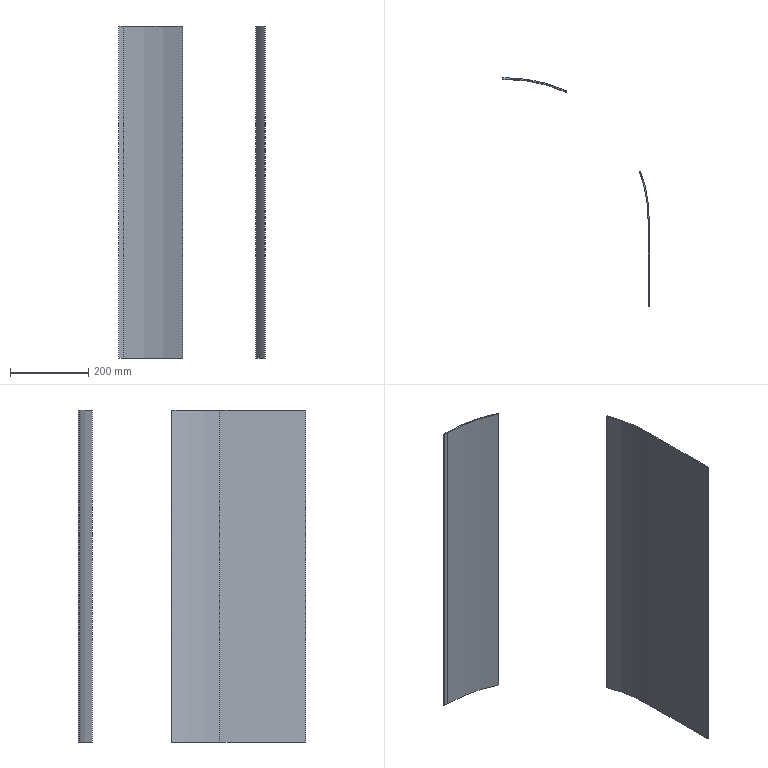Part | NX | features BREP 2, DATUM_CSYS 1, SKETCH 1 | 2 solids | 16 faces | box 375 x 583 x 850 mm | volume 1310584 mm3 | plane 12 | cylinder 4 | commonest cylinder face diameters 720 x2 726 x2
STEP:
#1=CARTESIAN_POINT('',(1041.108,124.153,-31.));
#2=VERTEX_POINT('',#1);
#3=CARTESIAN_POINT('',(1041.108,124.153,819.));
#4=VERTEX_POINT('',#3);
#5=CARTESIAN_POINT('',(1041.108,124.153,-31.));
#6=DIRECTION('',(0.,0.,1.));
#7=VECTOR('',#6,1000.);
#8=LINE('',#5,#7);
#9=EDGE_CURVE('',#2,#4,#8,.T.);
#10=ORIENTED_EDGE('',*,*,#9,.T.);
#11=CARTESIAN_POINT('',(1063.,0.,819.));
#12=VERTEX_POINT('',#11);
#13=CARTESIAN_POINT('',(700.,0.,819.));
#14=DIRECTION('',(0.,0.,-1.));
#15=DIRECTION('',(1.,0.,0.));
#16=AXIS2_PLACEMENT_3D('',#13,#14,#15);
#17=CIRCLE('',#16,363.);
#18=EDGE_CURVE('',#4,#12,#17,.T.);
#19=ORIENTED_EDGE('',*,*,#18,.T.);
#20=CARTESIAN_POINT('',(1063.,0.,-31.));
#21=VERTEX_POINT('',#20);
#22=CARTESIAN_POINT('',(1063.,0.,819.));
#23=DIRECTION('',(0.,0.,-1.));
#24=VECTOR('',#23,1000.);
#25=LINE('',#22,#24);
#26=EDGE_CURVE('',#12,#21,#25,.T.);
#27=ORIENTED_EDGE('',*,*,#26,.T.);
#28=CARTESIAN_POINT('',(700.,0.,-31.));
#29=DIRECTION('',(0.,0.,-1.));
#30=DIRECTION('',(1.,0.,0.));
#31=AXIS2_PLACEMENT_3D('',#28,#29,#30);
#32=CIRCLE('',#31,363.);
#33=EDGE_CURVE('',#2,#21,#32,.T.);
#34=ORIENTED_EDGE('',*,*,#33,.F.);
#35=EDGE_LOOP('',(#10,#19,#27,#34));
#36=FACE_BOUND('',#35,.T.);
#37=CARTESIAN_POINT('',(700.,0.,819.));
#38=DIRECTION('',(0.,0.,-1.));
#39=DIRECTION('',(1.,0.,0.));
#40=AXIS2_PLACEMENT_3D('',#37,#38,#39);
#41=CYLINDRICAL_SURFACE('',#40,363.);
#42=ADVANCED_FACE('',(#36),#41,.T.);
#43=CARTESIAN_POINT('',(1038.289,123.127,819.));
#44=VERTEX_POINT('',#43);
#45=CARTESIAN_POINT('',(1060.,0.,819.));
#46=VERTEX_POINT('',#45);
#47=CARTESIAN_POINT('',(700.,0.,819.));
#48=DIRECTION('',(0.,0.,-1.));
#49=DIRECTION('',(1.,0.,0.));
#50=AXIS2_PLACEMENT_3D('',#47,#48,#49);
#51=CIRCLE('',#50,360.);
#52=EDGE_CURVE('',#44,#46,#51,.T.);
#53=ORIENTED_EDGE('',*,*,#52,.F.);
#54=CARTESIAN_POINT('',(1038.289,123.127,-31.));
#55=VERTEX_POINT('',#54);
#56=CARTESIAN_POINT('',(1038.289,123.127,-31.));
#57=DIRECTION('',(0.,0.,1.));
#58=VECTOR('',#57,1000.);
#59=LINE('',#56,#58);
#60=EDGE_CURVE('',#55,#44,#59,.T.);
#61=ORIENTED_EDGE('',*,*,#60,.F.);
#62=CARTESIAN_POINT('',(1060.,0.,-31.));
#63=VERTEX_POINT('',#62);
#64=CARTESIAN_POINT('',(700.,0.,-31.));
#65=DIRECTION('',(0.,0.,-1.));
#66=DIRECTION('',(1.,0.,0.));
#67=AXIS2_PLACEMENT_3D('',#64,#65,#66);
#68=CIRCLE('',#67,360.);
#69=EDGE_CURVE('',#55,#63,#68,.T.);
#70=ORIENTED_EDGE('',*,*,#69,.T.);
#71=CARTESIAN_POINT('',(1060.,0.,819.));
#72=DIRECTION('',(0.,0.,-1.));
#73=VECTOR('',#72,1000.);
#74=LINE('',#71,#73);
#75=EDGE_CURVE('',#46,#63,#74,.T.);
#76=ORIENTED_EDGE('',*,*,#75,.F.);
#77=EDGE_LOOP('',(#53,#61,#70,#76));
#78=FACE_BOUND('',#77,.T.);
#79=CARTESIAN_POINT('',(700.,0.,819.));
#80=DIRECTION('',(0.,0.,-1.));
#81=DIRECTION('',(1.,0.,0.));
#82=AXIS2_PLACEMENT_3D('',#79,#80,#81);
#83=CYLINDRICAL_SURFACE('',#82,360.);
#84=ADVANCED_FACE('',(#78),#83,.F.);
#85=CARTESIAN_POINT('',(1041.108,124.153,819.));
#86=DIRECTION('',(0.9397,0.342,0.));
#87=VECTOR('',#86,1000.);
#88=LINE('',#85,#87);
#89=EDGE_CURVE('',#44,#4,#88,.T.);
#90=ORIENTED_EDGE('',*,*,#89,.F.);
#91=ORIENTED_EDGE('',*,*,#52,.T.);
#92=CARTESIAN_POINT('',(1060.,-220.,819.));
#93=VERTEX_POINT('',#92);
#94=CARTESIAN_POINT('',(1060.,0.,819.));
#95=DIRECTION('',(0.,-1.,0.));
#96=VECTOR('',#95,1000.);
#97=LINE('',#94,#96);
#98=EDGE_CURVE('',#46,#93,#97,.T.);
#99=ORIENTED_EDGE('',*,*,#98,.T.);
#100=CARTESIAN_POINT('',(1063.,-220.,819.));
#101=VERTEX_POINT('',#100);
#102=CARTESIAN_POINT('',(1063.,-220.,819.));
#103=DIRECTION('',(-1.,0.,0.));
#104=VECTOR('',#103,1000.);
#105=LINE('',#102,#104);
#106=EDGE_CURVE('',#101,#93,#105,.T.);
#107=ORIENTED_EDGE('',*,*,#106,.F.);
#108=CARTESIAN_POINT('',(1063.,0.,819.));
#109=DIRECTION('',(0.,-1.,0.));
#110=VECTOR('',#109,1000.);
#111=LINE('',#108,#110);
#112=EDGE_CURVE('',#12,#101,#111,.T.);
#113=ORIENTED_EDGE('',*,*,#112,.F.);
#114=ORIENTED_EDGE('',*,*,#18,.F.);
#115=EDGE_LOOP('',(#90,#91,#99,#107,#113,#114));
#116=FACE_BOUND('',#115,.T.);
#117=CARTESIAN_POINT('',(700.,0.,819.));
#118=DIRECTION('',(0.,0.,1.));
#119=DIRECTION('',(-1.,0.,0.));
#120=AXIS2_PLACEMENT_3D('',#117,#118,#119);
#121=PLANE('',#120);
#122=ADVANCED_FACE('',(#116),#121,.T.);
#123=ORIENTED_EDGE('',*,*,#69,.F.);
#124=CARTESIAN_POINT('',(1041.108,124.153,-31.));
#125=DIRECTION('',(0.9397,0.342,0.));
#126=VECTOR('',#125,1000.);
#127=LINE('',#124,#126);
#128=EDGE_CURVE('',#55,#2,#127,.T.);
#129=ORIENTED_EDGE('',*,*,#128,.T.);
#130=ORIENTED_EDGE('',*,*,#33,.T.);
#131=CARTESIAN_POINT('',(1063.,-220.,-31.));
#132=VERTEX_POINT('',#131);
#133=CARTESIAN_POINT('',(1063.,0.,-31.));
#134=DIRECTION('',(0.,-1.,0.));
#135=VECTOR('',#134,1000.);
#136=LINE('',#133,#135);
#137=EDGE_CURVE('',#21,#132,#136,.T.);
#138=ORIENTED_EDGE('',*,*,#137,.T.);
#139=CARTESIAN_POINT('',(1060.,-220.,-31.));
#140=VERTEX_POINT('',#139);
#141=CARTESIAN_POINT('',(1063.,-220.,-31.));
#142=DIRECTION('',(-1.,0.,0.));
#143=VECTOR('',#142,1000.);
#144=LINE('',#141,#143);
#145=EDGE_CURVE('',#132,#140,#144,.T.);
#146=ORIENTED_EDGE('',*,*,#145,.T.);
#147=CARTESIAN_POINT('',(1060.,0.,-31.));
#148=DIRECTION('',(0.,-1.,0.));
#149=VECTOR('',#148,1000.);
#150=LINE('',#147,#149);
#151=EDGE_CURVE('',#63,#140,#150,.T.);
#152=ORIENTED_EDGE('',*,*,#151,.F.);
#153=EDGE_LOOP('',(#123,#129,#130,#138,#146,#152));
#154=FACE_BOUND('',#153,.T.);
#155=CARTESIAN_POINT('',(700.,0.,-31.));
#156=DIRECTION('',(0.,0.,1.));
#157=DIRECTION('',(-1.,0.,0.));
#158=AXIS2_PLACEMENT_3D('',#155,#156,#157);
#159=PLANE('',#158);
#160=ADVANCED_FACE('',(#154),#159,.F.);
#161=ORIENTED_EDGE('',*,*,#151,.T.);
#162=CARTESIAN_POINT('',(1060.,-220.,819.));
#163=DIRECTION('',(0.,0.,-1.));
#164=VECTOR('',#163,1000.);
#165=LINE('',#162,#164);
#166=EDGE_CURVE('',#93,#140,#165,.T.);
#167=ORIENTED_EDGE('',*,*,#166,.F.);
#168=ORIENTED_EDGE('',*,*,#98,.F.);
#169=ORIENTED_EDGE('',*,*,#75,.T.);
#170=EDGE_LOOP('',(#161,#167,#168,#169));
#171=FACE_BOUND('',#170,.T.);
#172=CARTESIAN_POINT('',(1060.,0.,819.));
#173=DIRECTION('',(1.,0.,0.));
#174=DIRECTION('',(0.,0.,1.));
#175=AXIS2_PLACEMENT_3D('',#172,#173,#174);
#176=PLANE('',#175);
#177=ADVANCED_FACE('',(#171),#176,.F.);
#178=ORIENTED_EDGE('',*,*,#145,.F.);
#179=CARTESIAN_POINT('',(1063.,-220.,819.));
#180=DIRECTION('',(0.,0.,-1.));
#181=VECTOR('',#180,1000.);
#182=LINE('',#179,#181);
#183=EDGE_CURVE('',#101,#132,#182,.T.);
#184=ORIENTED_EDGE('',*,*,#183,.F.);
#185=ORIENTED_EDGE('',*,*,#106,.T.);
#186=ORIENTED_EDGE('',*,*,#166,.T.);
#187=EDGE_LOOP('',(#178,#184,#185,#186));
#188=FACE_BOUND('',#187,.T.);
#189=CARTESIAN_POINT('',(1063.,-220.,819.));
#190=DIRECTION('',(0.,-1.,0.));
#191=DIRECTION('',(0.,0.,1.));
#192=AXIS2_PLACEMENT_3D('',#189,#190,#191);
#193=PLANE('',#192);
#194=ADVANCED_FACE('',(#188),#193,.T.);
#195=ORIENTED_EDGE('',*,*,#137,.F.);
#196=ORIENTED_EDGE('',*,*,#26,.F.);
#197=ORIENTED_EDGE('',*,*,#112,.T.);
#198=ORIENTED_EDGE('',*,*,#183,.T.);
#199=EDGE_LOOP('',(#195,#196,#197,#198));
#200=FACE_BOUND('',#199,.T.);
#201=CARTESIAN_POINT('',(1063.,0.,819.));
#202=DIRECTION('',(1.,0.,0.));
#203=DIRECTION('',(0.,0.,1.));
#204=AXIS2_PLACEMENT_3D('',#201,#202,#203);
#205=PLANE('',#204);
#206=ADVANCED_FACE('',(#200),#205,.T.);
#207=ORIENTED_EDGE('',*,*,#89,.T.);
#208=ORIENTED_EDGE('',*,*,#9,.F.);
#209=ORIENTED_EDGE('',*,*,#128,.F.);
#210=ORIENTED_EDGE('',*,*,#60,.T.);
#211=EDGE_LOOP('',(#207,#208,#209,#210));
#212=FACE_BOUND('',#211,.T.);
#213=CARTESIAN_POINT('',(1041.108,124.153,-31.));
#214=DIRECTION('',(0.342,-0.9397,0.));
#215=DIRECTION('',(-0.9397,-0.342,0.));
#216=AXIS2_PLACEMENT_3D('',#213,#214,#215);
#217=PLANE('',#216);
#218=ADVANCED_FACE('',(#212),#217,.F.);
#219=CLOSED_SHELL('',(#42,#84,#122,#160,#177,#194,#206,#218));
#220=MANIFOLD_SOLID_BREP('',#219);
#221=CARTESIAN_POINT('',(688.,363.,-31.));
#222=VERTEX_POINT('',#221);
#223=CARTESIAN_POINT('',(700.,363.,-31.));
#224=VERTEX_POINT('',#223);
#225=CARTESIAN_POINT('',(700.,363.,-31.));
#226=DIRECTION('',(1.,0.,0.));
#227=VECTOR('',#226,1000.);
#228=LINE('',#225,#227);
#229=EDGE_CURVE('',#222,#224,#228,.T.);
#230=ORIENTED_EDGE('',*,*,#229,.F.);
#231=CARTESIAN_POINT('',(688.,363.,819.));
#232=VERTEX_POINT('',#231);
#233=CARTESIAN_POINT('',(688.,363.,819.));
#234=DIRECTION('',(0.,0.,-1.));
#235=VECTOR('',#234,1000.);
#236=LINE('',#233,#235);
#237=EDGE_CURVE('',#232,#222,#236,.T.);
#238=ORIENTED_EDGE('',*,*,#237,.F.);
#239=CARTESIAN_POINT('',(700.,363.,819.));
#240=VERTEX_POINT('',#239);
#241=CARTESIAN_POINT('',(700.,363.,819.));
#242=DIRECTION('',(1.,0.,0.));
#243=VECTOR('',#242,1000.);
#244=LINE('',#241,#243);
#245=EDGE_CURVE('',#232,#240,#244,.T.);
#246=ORIENTED_EDGE('',*,*,#245,.T.);
#247=CARTESIAN_POINT('',(700.,363.,819.));
#248=DIRECTION('',(0.,0.,-1.));
#249=VECTOR('',#248,1000.);
#250=LINE('',#247,#249);
#251=EDGE_CURVE('',#240,#224,#250,.T.);
#252=ORIENTED_EDGE('',*,*,#251,.T.);
#253=EDGE_LOOP('',(#230,#238,#246,#252));
#254=FACE_BOUND('',#253,.T.);
#255=CARTESIAN_POINT('',(700.,363.,819.));
#256=DIRECTION('',(0.,1.,0.));
#257=DIRECTION('',(1.,0.,0.));
#258=AXIS2_PLACEMENT_3D('',#255,#256,#257);
#259=PLANE('',#258);
#260=ADVANCED_FACE('',(#254),#259,.T.);
#261=CARTESIAN_POINT('',(688.,360.,-31.));
#262=VERTEX_POINT('',#261);
#263=CARTESIAN_POINT('',(688.,360.,-31.));
#264=DIRECTION('',(0.,1.,0.));
#265=VECTOR('',#264,1000.);
#266=LINE('',#263,#265);
#267=EDGE_CURVE('',#262,#222,#266,.T.);
#268=ORIENTED_EDGE('',*,*,#267,.F.);
#269=CARTESIAN_POINT('',(688.,360.,819.));
#270=VERTEX_POINT('',#269);
#271=CARTESIAN_POINT('',(688.,360.,819.));
#272=DIRECTION('',(0.,0.,-1.));
#273=VECTOR('',#272,1000.);
#274=LINE('',#271,#273);
#275=EDGE_CURVE('',#270,#262,#274,.T.);
#276=ORIENTED_EDGE('',*,*,#275,.F.);
#277=CARTESIAN_POINT('',(688.,360.,819.));
#278=DIRECTION('',(0.,1.,0.));
#279=VECTOR('',#278,1000.);
#280=LINE('',#277,#279);
#281=EDGE_CURVE('',#270,#232,#280,.T.);
#282=ORIENTED_EDGE('',*,*,#281,.T.);
#283=ORIENTED_EDGE('',*,*,#237,.T.);
#284=EDGE_LOOP('',(#268,#276,#282,#283));
#285=FACE_BOUND('',#284,.T.);
#286=CARTESIAN_POINT('',(688.,360.,819.));
#287=DIRECTION('',(-1.,0.,0.));
#288=DIRECTION('',(0.,0.,-1.));
#289=AXIS2_PLACEMENT_3D('',#286,#287,#288);
#290=PLANE('',#289);
#291=ADVANCED_FACE('',(#285),#290,.T.);
#292=CARTESIAN_POINT('',(700.,360.,-31.));
#293=VERTEX_POINT('',#292);
#294=CARTESIAN_POINT('',(700.,360.,-31.));
#295=DIRECTION('',(1.,0.,0.));
#296=VECTOR('',#295,1000.);
#297=LINE('',#294,#296);
#298=EDGE_CURVE('',#262,#293,#297,.T.);
#299=ORIENTED_EDGE('',*,*,#298,.T.);
#300=CARTESIAN_POINT('',(700.,360.,819.));
#301=VERTEX_POINT('',#300);
#302=CARTESIAN_POINT('',(700.,360.,819.));
#303=DIRECTION('',(0.,0.,-1.));
#304=VECTOR('',#303,1000.);
#305=LINE('',#302,#304);
#306=EDGE_CURVE('',#301,#293,#305,.T.);
#307=ORIENTED_EDGE('',*,*,#306,.F.);
#308=CARTESIAN_POINT('',(700.,360.,819.));
#309=DIRECTION('',(1.,0.,0.));
#310=VECTOR('',#309,1000.);
#311=LINE('',#308,#310);
#312=EDGE_CURVE('',#270,#301,#311,.T.);
#313=ORIENTED_EDGE('',*,*,#312,.F.);
#314=ORIENTED_EDGE('',*,*,#275,.T.);
#315=EDGE_LOOP('',(#299,#307,#313,#314));
#316=FACE_BOUND('',#315,.T.);
#317=CARTESIAN_POINT('',(700.,360.,819.));
#318=DIRECTION('',(0.,1.,0.));
#319=DIRECTION('',(1.,0.,0.));
#320=AXIS2_PLACEMENT_3D('',#317,#318,#319);
#321=PLANE('',#320);
#322=ADVANCED_FACE('',(#316),#321,.F.);
#323=CARTESIAN_POINT('',(851.618,329.82,819.));
#324=VERTEX_POINT('',#323);
#325=CARTESIAN_POINT('',(850.365,327.094,819.));
#326=VERTEX_POINT('',#325);
#327=CARTESIAN_POINT('',(851.618,329.82,819.));
#328=DIRECTION('',(-0.4177,-0.9086,0.));
#329=VECTOR('',#328,1000.);
#330=LINE('',#327,#329);
#331=EDGE_CURVE('',#324,#326,#330,.T.);
#332=ORIENTED_EDGE('',*,*,#331,.F.);
#333=CARTESIAN_POINT('',(700.,0.,819.));
#334=DIRECTION('',(0.,0.,-1.));
#335=DIRECTION('',(1.,0.,0.));
#336=AXIS2_PLACEMENT_3D('',#333,#334,#335);
#337=CIRCLE('',#336,363.);
#338=EDGE_CURVE('',#240,#324,#337,.T.);
#339=ORIENTED_EDGE('',*,*,#338,.F.);
#340=ORIENTED_EDGE('',*,*,#245,.F.);
#341=ORIENTED_EDGE('',*,*,#281,.F.);
#342=ORIENTED_EDGE('',*,*,#312,.T.);
#343=CARTESIAN_POINT('',(700.,0.,819.));
#344=DIRECTION('',(0.,0.,-1.));
#345=DIRECTION('',(1.,0.,0.));
#346=AXIS2_PLACEMENT_3D('',#343,#344,#345);
#347=CIRCLE('',#346,360.);
#348=EDGE_CURVE('',#301,#326,#347,.T.);
#349=ORIENTED_EDGE('',*,*,#348,.T.);
#350=EDGE_LOOP('',(#332,#339,#340,#341,#342,#349));
#351=FACE_BOUND('',#350,.T.);
#352=CARTESIAN_POINT('',(700.,0.,819.));
#353=DIRECTION('',(0.,0.,1.));
#354=DIRECTION('',(-1.,0.,0.));
#355=AXIS2_PLACEMENT_3D('',#352,#353,#354);
#356=PLANE('',#355);
#357=ADVANCED_FACE('',(#351),#356,.T.);
#358=CARTESIAN_POINT('',(851.618,329.82,-31.));
#359=VERTEX_POINT('',#358);
#360=CARTESIAN_POINT('',(700.,0.,-31.));
#361=DIRECTION('',(0.,0.,-1.));
#362=DIRECTION('',(1.,0.,0.));
#363=AXIS2_PLACEMENT_3D('',#360,#361,#362);
#364=CIRCLE('',#363,363.);
#365=EDGE_CURVE('',#224,#359,#364,.T.);
#366=ORIENTED_EDGE('',*,*,#365,.T.);
#367=CARTESIAN_POINT('',(850.365,327.094,-31.));
#368=VERTEX_POINT('',#367);
#369=CARTESIAN_POINT('',(851.618,329.82,-31.));
#370=DIRECTION('',(-0.4177,-0.9086,0.));
#371=VECTOR('',#370,1000.);
#372=LINE('',#369,#371);
#373=EDGE_CURVE('',#359,#368,#372,.T.);
#374=ORIENTED_EDGE('',*,*,#373,.T.);
#375=CARTESIAN_POINT('',(700.,0.,-31.));
#376=DIRECTION('',(0.,0.,-1.));
#377=DIRECTION('',(1.,0.,0.));
#378=AXIS2_PLACEMENT_3D('',#375,#376,#377);
#379=CIRCLE('',#378,360.);
#380=EDGE_CURVE('',#293,#368,#379,.T.);
#381=ORIENTED_EDGE('',*,*,#380,.F.);
#382=ORIENTED_EDGE('',*,*,#298,.F.);
#383=ORIENTED_EDGE('',*,*,#267,.T.);
#384=ORIENTED_EDGE('',*,*,#229,.T.);
#385=EDGE_LOOP('',(#366,#374,#381,#382,#383,#384));
#386=FACE_BOUND('',#385,.T.);
#387=CARTESIAN_POINT('',(700.,0.,-31.));
#388=DIRECTION('',(0.,0.,1.));
#389=DIRECTION('',(-1.,0.,0.));
#390=AXIS2_PLACEMENT_3D('',#387,#388,#389);
#391=PLANE('',#390);
#392=ADVANCED_FACE('',(#386),#391,.F.);
#393=ORIENTED_EDGE('',*,*,#380,.T.);
#394=CARTESIAN_POINT('',(850.365,327.094,-31.));
#395=DIRECTION('',(0.,0.,1.));
#396=VECTOR('',#395,1000.);
#397=LINE('',#394,#396);
#398=EDGE_CURVE('',#368,#326,#397,.T.);
#399=ORIENTED_EDGE('',*,*,#398,.T.);
#400=ORIENTED_EDGE('',*,*,#348,.F.);
#401=ORIENTED_EDGE('',*,*,#306,.T.);
#402=EDGE_LOOP('',(#393,#399,#400,#401));
#403=FACE_BOUND('',#402,.T.);
#404=CARTESIAN_POINT('',(700.,0.,819.));
#405=DIRECTION('',(0.,0.,-1.));
#406=DIRECTION('',(1.,0.,0.));
#407=AXIS2_PLACEMENT_3D('',#404,#405,#406);
#408=CYLINDRICAL_SURFACE('',#407,360.);
#409=ADVANCED_FACE('',(#403),#408,.F.);
#410=CARTESIAN_POINT('',(851.618,329.82,-31.));
#411=DIRECTION('',(0.,0.,1.));
#412=VECTOR('',#411,1000.);
#413=LINE('',#410,#412);
#414=EDGE_CURVE('',#359,#324,#413,.T.);
#415=ORIENTED_EDGE('',*,*,#414,.F.);
#416=ORIENTED_EDGE('',*,*,#365,.F.);
#417=ORIENTED_EDGE('',*,*,#251,.F.);
#418=ORIENTED_EDGE('',*,*,#338,.T.);
#419=EDGE_LOOP('',(#415,#416,#417,#418));
#420=FACE_BOUND('',#419,.T.);
#421=CARTESIAN_POINT('',(700.,0.,819.));
#422=DIRECTION('',(0.,0.,-1.));
#423=DIRECTION('',(1.,0.,0.));
#424=AXIS2_PLACEMENT_3D('',#421,#422,#423);
#425=CYLINDRICAL_SURFACE('',#424,363.);
#426=ADVANCED_FACE('',(#420),#425,.T.);
#427=ORIENTED_EDGE('',*,*,#331,.T.);
#428=ORIENTED_EDGE('',*,*,#398,.F.);
#429=ORIENTED_EDGE('',*,*,#373,.F.);
#430=ORIENTED_EDGE('',*,*,#414,.T.);
#431=EDGE_LOOP('',(#427,#428,#429,#430));
#432=FACE_BOUND('',#431,.T.);
#433=CARTESIAN_POINT('',(851.618,329.82,-31.));
#434=DIRECTION('',(-0.9086,0.4177,0.));
#435=DIRECTION('',(0.4177,0.9086,0.));
#436=AXIS2_PLACEMENT_3D('',#433,#434,#435);
#437=PLANE('',#436);
#438=ADVANCED_FACE('',(#432),#437,.F.);
#439=CLOSED_SHELL('',(#260,#291,#322,#357,#392,#409,#426,#438));
#440=MANIFOLD_SOLID_BREP('',#439);
#441=(LENGTH_UNIT()NAMED_UNIT(*)SI_UNIT(.MILLI.,.METRE.));
#442=UNCERTAINTY_MEASURE_WITH_UNIT(LENGTH_MEASURE(0.00001),#441,'','');
#443=(NAMED_UNIT(*)PLANE_ANGLE_UNIT()SI_UNIT($,.RADIAN.));
#444=(NAMED_UNIT(*)SI_UNIT($,.STERADIAN.)SOLID_ANGLE_UNIT());
#445=(GEOMETRIC_REPRESENTATION_CONTEXT(3)GLOBAL_UNCERTAINTY_ASSIGNED_CONTEXT((#442))GLOBAL_UNIT_ASSIGNED_CONTEXT((#441,#443,#444))REPRESENTATION_CONTEXT('',''));
#446=ADVANCED_BREP_SHAPE_REPRESENTATION('',(#220,#440),#445);